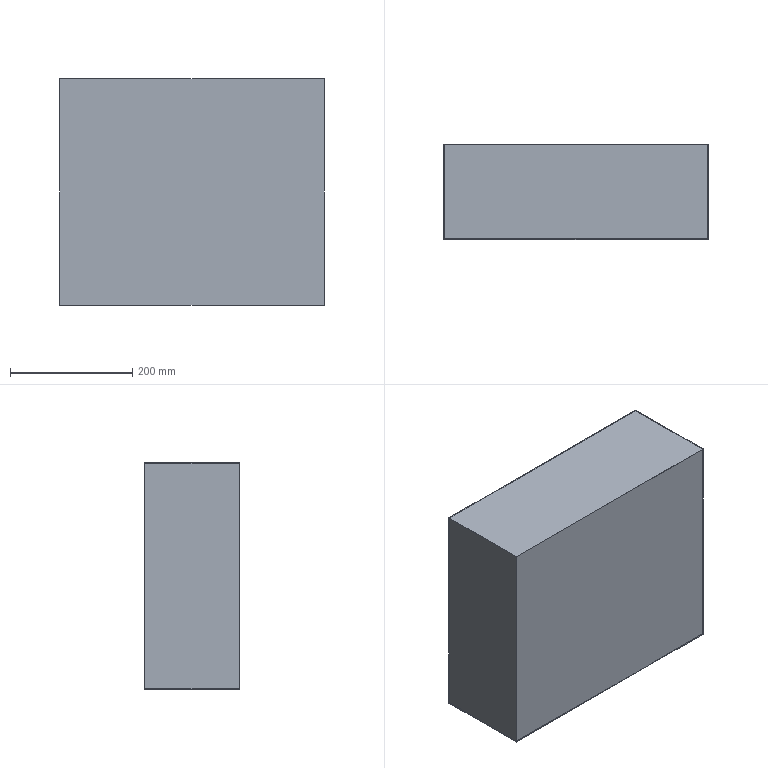Part | STEP file | STANDARD CONTRILLER | 1 solid | 12 faces | box 432 x 156 x 371 mm | volume 567252 mm3 | plane 12
STEP:
#1=CARTESIAN_POINT('',(-70.587,137.128,371.));
#2=VERTEX_POINT('',#1);
#3=CARTESIAN_POINT('',(-70.587,-18.872,371.));
#4=VERTEX_POINT('',#3);
#5=CARTESIAN_POINT('',(-70.587,136.128,371.));
#6=DIRECTION('',(0.,-1.,0.));
#7=VECTOR('',#6,1000.);
#8=LINE('',#5,#7);
#9=EDGE_CURVE('',#2,#4,#8,.T.);
#10=ORIENTED_EDGE('',*,*,#9,.T.);
#11=CARTESIAN_POINT('',(361.413,-18.872,371.));
#12=VERTEX_POINT('',#11);
#13=CARTESIAN_POINT('',(-69.587,-18.872,371.));
#14=DIRECTION('',(1.,0.,0.));
#15=VECTOR('',#14,1000.);
#16=LINE('',#13,#15);
#17=EDGE_CURVE('',#4,#12,#16,.T.);
#18=ORIENTED_EDGE('',*,*,#17,.T.);
#19=CARTESIAN_POINT('',(361.413,137.128,371.));
#20=VERTEX_POINT('',#19);
#21=CARTESIAN_POINT('',(361.413,136.128,371.));
#22=DIRECTION('',(0.,1.,0.));
#23=VECTOR('',#22,1000.);
#24=LINE('',#21,#23);
#25=EDGE_CURVE('',#12,#20,#24,.T.);
#26=ORIENTED_EDGE('',*,*,#25,.T.);
#27=CARTESIAN_POINT('',(-69.587,137.128,371.));
#28=DIRECTION('',(-1.,0.,0.));
#29=VECTOR('',#28,1000.);
#30=LINE('',#27,#29);
#31=EDGE_CURVE('',#20,#2,#30,.T.);
#32=ORIENTED_EDGE('',*,*,#31,.T.);
#33=EDGE_LOOP('',(#10,#18,#26,#32));
#34=FACE_OUTER_BOUND('',#33,.T.);
#35=CARTESIAN_POINT('',(-70.587,-18.872,371.));
#36=DIRECTION('',(0.,0.,1.));
#37=DIRECTION('',(1.,0.,0.));
#38=AXIS2_PLACEMENT_3D('',#35,#36,#37);
#39=PLANE('',#38);
#40=ADVANCED_FACE('',(#34),#39,.T.);
#41=CARTESIAN_POINT('',(-70.587,137.128,0.));
#42=VERTEX_POINT('',#41);
#43=CARTESIAN_POINT('',(-70.587,-18.872,0.));
#44=VERTEX_POINT('',#43);
#45=CARTESIAN_POINT('',(-70.587,136.128,0.));
#46=DIRECTION('',(0.,-1.,0.));
#47=VECTOR('',#46,1000.);
#48=LINE('',#45,#47);
#49=EDGE_CURVE('',#42,#44,#48,.T.);
#50=ORIENTED_EDGE('',*,*,#49,.F.);
#51=CARTESIAN_POINT('',(361.413,137.128,0.));
#52=VERTEX_POINT('',#51);
#53=CARTESIAN_POINT('',(-69.587,137.128,0.));
#54=DIRECTION('',(-1.,0.,0.));
#55=VECTOR('',#54,1000.);
#56=LINE('',#53,#55);
#57=EDGE_CURVE('',#52,#42,#56,.T.);
#58=ORIENTED_EDGE('',*,*,#57,.F.);
#59=CARTESIAN_POINT('',(361.413,-18.872,0.));
#60=VERTEX_POINT('',#59);
#61=CARTESIAN_POINT('',(361.413,136.128,0.));
#62=DIRECTION('',(0.,1.,0.));
#63=VECTOR('',#62,1000.);
#64=LINE('',#61,#63);
#65=EDGE_CURVE('',#60,#52,#64,.T.);
#66=ORIENTED_EDGE('',*,*,#65,.F.);
#67=CARTESIAN_POINT('',(-69.587,-18.872,0.));
#68=DIRECTION('',(1.,0.,0.));
#69=VECTOR('',#68,1000.);
#70=LINE('',#67,#69);
#71=EDGE_CURVE('',#44,#60,#70,.T.);
#72=ORIENTED_EDGE('',*,*,#71,.F.);
#73=EDGE_LOOP('',(#50,#58,#66,#72));
#74=FACE_OUTER_BOUND('',#73,.T.);
#75=CARTESIAN_POINT('',(-70.587,-18.872,0.));
#76=DIRECTION('',(0.,0.,1.));
#77=DIRECTION('',(1.,0.,0.));
#78=AXIS2_PLACEMENT_3D('',#75,#76,#77);
#79=PLANE('',#78);
#80=ADVANCED_FACE('',(#74),#79,.F.);
#81=ORIENTED_EDGE('',*,*,#49,.T.);
#82=CARTESIAN_POINT('',(-70.587,-18.872,371.));
#83=DIRECTION('',(0.,0.,-1.));
#84=VECTOR('',#83,1000.);
#85=LINE('',#82,#84);
#86=EDGE_CURVE('',#4,#44,#85,.T.);
#87=ORIENTED_EDGE('',*,*,#86,.F.);
#88=ORIENTED_EDGE('',*,*,#9,.F.);
#89=CARTESIAN_POINT('',(-70.587,137.128,371.));
#90=DIRECTION('',(0.,0.,-1.));
#91=VECTOR('',#90,1000.);
#92=LINE('',#89,#91);
#93=EDGE_CURVE('',#2,#42,#92,.T.);
#94=ORIENTED_EDGE('',*,*,#93,.T.);
#95=EDGE_LOOP('',(#81,#87,#88,#94));
#96=FACE_OUTER_BOUND('',#95,.T.);
#97=CARTESIAN_POINT('',(-70.587,136.128,371.));
#98=DIRECTION('',(1.,0.,0.));
#99=DIRECTION('',(0.,1.,0.));
#100=AXIS2_PLACEMENT_3D('',#97,#98,#99);
#101=PLANE('',#100);
#102=ADVANCED_FACE('',(#96),#101,.F.);
#103=ORIENTED_EDGE('',*,*,#71,.T.);
#104=CARTESIAN_POINT('',(361.413,-18.872,371.));
#105=DIRECTION('',(0.,0.,-1.));
#106=VECTOR('',#105,1000.);
#107=LINE('',#104,#106);
#108=EDGE_CURVE('',#12,#60,#107,.T.);
#109=ORIENTED_EDGE('',*,*,#108,.F.);
#110=ORIENTED_EDGE('',*,*,#17,.F.);
#111=ORIENTED_EDGE('',*,*,#86,.T.);
#112=EDGE_LOOP('',(#103,#109,#110,#111));
#113=FACE_OUTER_BOUND('',#112,.T.);
#114=CARTESIAN_POINT('',(-69.587,-18.872,371.));
#115=DIRECTION('',(0.,1.,0.));
#116=DIRECTION('',(0.,0.,1.));
#117=AXIS2_PLACEMENT_3D('',#114,#115,#116);
#118=PLANE('',#117);
#119=ADVANCED_FACE('',(#113),#118,.F.);
#120=ORIENTED_EDGE('',*,*,#65,.T.);
#121=CARTESIAN_POINT('',(361.413,137.128,371.));
#122=DIRECTION('',(0.,0.,-1.));
#123=VECTOR('',#122,1000.);
#124=LINE('',#121,#123);
#125=EDGE_CURVE('',#20,#52,#124,.T.);
#126=ORIENTED_EDGE('',*,*,#125,.F.);
#127=ORIENTED_EDGE('',*,*,#25,.F.);
#128=ORIENTED_EDGE('',*,*,#108,.T.);
#129=EDGE_LOOP('',(#120,#126,#127,#128));
#130=FACE_OUTER_BOUND('',#129,.T.);
#131=CARTESIAN_POINT('',(361.413,136.128,371.));
#132=DIRECTION('',(-1.,0.,0.));
#133=DIRECTION('',(0.,0.,1.));
#134=AXIS2_PLACEMENT_3D('',#131,#132,#133);
#135=PLANE('',#134);
#136=ADVANCED_FACE('',(#130),#135,.F.);
#137=ORIENTED_EDGE('',*,*,#57,.T.);
#138=ORIENTED_EDGE('',*,*,#93,.F.);
#139=ORIENTED_EDGE('',*,*,#31,.F.);
#140=ORIENTED_EDGE('',*,*,#125,.T.);
#141=EDGE_LOOP('',(#137,#138,#139,#140));
#142=FACE_OUTER_BOUND('',#141,.T.);
#143=CARTESIAN_POINT('',(-69.587,137.128,371.));
#144=DIRECTION('',(0.,-1.,0.));
#145=DIRECTION('',(0.,0.,-1.));
#146=AXIS2_PLACEMENT_3D('',#143,#144,#145);
#147=PLANE('',#146);
#148=ADVANCED_FACE('',(#142),#147,.F.);
#149=CLOSED_SHELL('',(#40,#80,#102,#119,#136,#148));
#150=CARTESIAN_POINT('',(360.413,136.128,1.));
#151=VERTEX_POINT('',#150);
#152=CARTESIAN_POINT('',(360.413,-17.872,1.));
#153=VERTEX_POINT('',#152);
#154=CARTESIAN_POINT('',(360.413,136.128,1.));
#155=DIRECTION('',(0.,-1.,0.));
#156=VECTOR('',#155,1000.);
#157=LINE('',#154,#156);
#158=EDGE_CURVE('',#151,#153,#157,.T.);
#159=ORIENTED_EDGE('',*,*,#158,.F.);
#160=CARTESIAN_POINT('',(-69.587,136.128,1.));
#161=VERTEX_POINT('',#160);
#162=CARTESIAN_POINT('',(360.413,136.128,1.));
#163=DIRECTION('',(1.,0.,0.));
#164=VECTOR('',#163,1000.);
#165=LINE('',#162,#164);
#166=EDGE_CURVE('',#161,#151,#165,.T.);
#167=ORIENTED_EDGE('',*,*,#166,.F.);
#168=CARTESIAN_POINT('',(-69.587,-17.872,1.));
#169=VERTEX_POINT('',#168);
#170=CARTESIAN_POINT('',(-69.587,136.128,1.));
#171=DIRECTION('',(0.,1.,0.));
#172=VECTOR('',#171,1000.);
#173=LINE('',#170,#172);
#174=EDGE_CURVE('',#169,#161,#173,.T.);
#175=ORIENTED_EDGE('',*,*,#174,.F.);
#176=CARTESIAN_POINT('',(360.413,-17.872,1.));
#177=DIRECTION('',(-1.,0.,0.));
#178=VECTOR('',#177,1000.);
#179=LINE('',#176,#178);
#180=EDGE_CURVE('',#153,#169,#179,.T.);
#181=ORIENTED_EDGE('',*,*,#180,.F.);
#182=EDGE_LOOP('',(#159,#167,#175,#181));
#183=FACE_OUTER_BOUND('',#182,.T.);
#184=CARTESIAN_POINT('',(360.413,-17.872,1.));
#185=DIRECTION('',(0.,0.,-1.));
#186=DIRECTION('',(-1.,0.,0.));
#187=AXIS2_PLACEMENT_3D('',#184,#185,#186);
#188=PLANE('',#187);
#189=ADVANCED_FACE('',(#183),#188,.F.);
#190=CARTESIAN_POINT('',(-69.587,136.128,370.));
#191=VERTEX_POINT('',#190);
#192=CARTESIAN_POINT('',(-69.587,-17.872,370.));
#193=VERTEX_POINT('',#192);
#194=CARTESIAN_POINT('',(-69.587,136.128,370.));
#195=DIRECTION('',(0.,-1.,0.));
#196=VECTOR('',#195,1000.);
#197=LINE('',#194,#196);
#198=EDGE_CURVE('',#191,#193,#197,.T.);
#199=ORIENTED_EDGE('',*,*,#198,.F.);
#200=CARTESIAN_POINT('',(360.413,136.128,370.));
#201=VERTEX_POINT('',#200);
#202=CARTESIAN_POINT('',(-69.587,136.128,370.));
#203=DIRECTION('',(-1.,0.,0.));
#204=VECTOR('',#203,1000.);
#205=LINE('',#202,#204);
#206=EDGE_CURVE('',#201,#191,#205,.T.);
#207=ORIENTED_EDGE('',*,*,#206,.F.);
#208=CARTESIAN_POINT('',(360.413,-17.872,370.));
#209=VERTEX_POINT('',#208);
#210=CARTESIAN_POINT('',(360.413,136.128,370.));
#211=DIRECTION('',(0.,1.,0.));
#212=VECTOR('',#211,1000.);
#213=LINE('',#210,#212);
#214=EDGE_CURVE('',#209,#201,#213,.T.);
#215=ORIENTED_EDGE('',*,*,#214,.F.);
#216=CARTESIAN_POINT('',(-69.587,-17.872,370.));
#217=DIRECTION('',(1.,0.,0.));
#218=VECTOR('',#217,1000.);
#219=LINE('',#216,#218);
#220=EDGE_CURVE('',#193,#209,#219,.T.);
#221=ORIENTED_EDGE('',*,*,#220,.F.);
#222=EDGE_LOOP('',(#199,#207,#215,#221));
#223=FACE_OUTER_BOUND('',#222,.T.);
#224=CARTESIAN_POINT('',(-69.587,-17.872,370.));
#225=DIRECTION('',(0.,0.,1.));
#226=DIRECTION('',(1.,0.,0.));
#227=AXIS2_PLACEMENT_3D('',#224,#225,#226);
#228=PLANE('',#227);
#229=ADVANCED_FACE('',(#223),#228,.F.);
#230=CARTESIAN_POINT('',(-69.587,136.128,371.));
#231=DIRECTION('',(0.,0.,-1.));
#232=VECTOR('',#231,1000.);
#233=LINE('',#230,#232);
#234=EDGE_CURVE('',#191,#161,#233,.T.);
#235=ORIENTED_EDGE('',*,*,#234,.T.);
#236=ORIENTED_EDGE('',*,*,#166,.T.);
#237=CARTESIAN_POINT('',(360.413,136.128,371.));
#238=DIRECTION('',(0.,0.,-1.));
#239=VECTOR('',#238,1000.);
#240=LINE('',#237,#239);
#241=EDGE_CURVE('',#201,#151,#240,.T.);
#242=ORIENTED_EDGE('',*,*,#241,.F.);
#243=ORIENTED_EDGE('',*,*,#206,.T.);
#244=EDGE_LOOP('',(#235,#236,#242,#243));
#245=FACE_OUTER_BOUND('',#244,.T.);
#246=CARTESIAN_POINT('',(-69.587,136.128,371.));
#247=DIRECTION('',(0.,-1.,0.));
#248=DIRECTION('',(0.,0.,-1.));
#249=AXIS2_PLACEMENT_3D('',#246,#247,#248);
#250=PLANE('',#249);
#251=ADVANCED_FACE('',(#245),#250,.T.);
#252=ORIENTED_EDGE('',*,*,#241,.T.);
#253=ORIENTED_EDGE('',*,*,#158,.T.);
#254=CARTESIAN_POINT('',(360.413,-17.872,371.));
#255=DIRECTION('',(0.,0.,-1.));
#256=VECTOR('',#255,1000.);
#257=LINE('',#254,#256);
#258=EDGE_CURVE('',#209,#153,#257,.T.);
#259=ORIENTED_EDGE('',*,*,#258,.F.);
#260=ORIENTED_EDGE('',*,*,#214,.T.);
#261=EDGE_LOOP('',(#252,#253,#259,#260));
#262=FACE_OUTER_BOUND('',#261,.T.);
#263=CARTESIAN_POINT('',(360.413,136.128,371.));
#264=DIRECTION('',(-1.,0.,0.));
#265=DIRECTION('',(0.,0.,1.));
#266=AXIS2_PLACEMENT_3D('',#263,#264,#265);
#267=PLANE('',#266);
#268=ADVANCED_FACE('',(#262),#267,.T.);
#269=ORIENTED_EDGE('',*,*,#258,.T.);
#270=ORIENTED_EDGE('',*,*,#180,.T.);
#271=CARTESIAN_POINT('',(-69.587,-17.872,371.));
#272=DIRECTION('',(0.,0.,-1.));
#273=VECTOR('',#272,1000.);
#274=LINE('',#271,#273);
#275=EDGE_CURVE('',#193,#169,#274,.T.);
#276=ORIENTED_EDGE('',*,*,#275,.F.);
#277=ORIENTED_EDGE('',*,*,#220,.T.);
#278=EDGE_LOOP('',(#269,#270,#276,#277));
#279=FACE_OUTER_BOUND('',#278,.T.);
#280=CARTESIAN_POINT('',(-69.587,-17.872,371.));
#281=DIRECTION('',(0.,1.,0.));
#282=DIRECTION('',(0.,0.,1.));
#283=AXIS2_PLACEMENT_3D('',#280,#281,#282);
#284=PLANE('',#283);
#285=ADVANCED_FACE('',(#279),#284,.T.);
#286=ORIENTED_EDGE('',*,*,#275,.T.);
#287=ORIENTED_EDGE('',*,*,#174,.T.);
#288=ORIENTED_EDGE('',*,*,#234,.F.);
#289=ORIENTED_EDGE('',*,*,#198,.T.);
#290=EDGE_LOOP('',(#286,#287,#288,#289));
#291=FACE_OUTER_BOUND('',#290,.T.);
#292=CARTESIAN_POINT('',(-69.587,136.128,371.));
#293=DIRECTION('',(1.,0.,0.));
#294=DIRECTION('',(0.,1.,0.));
#295=AXIS2_PLACEMENT_3D('',#292,#293,#294);
#296=PLANE('',#295);
#297=ADVANCED_FACE('',(#291),#296,.T.);
#298=CLOSED_SHELL('',(#189,#229,#251,#268,#285,#297));
#299=ORIENTED_CLOSED_SHELL('',*,#298,.F.);
#300=BREP_WITH_VOIDS('',#149,(#299));
#301=CARTESIAN_POINT('',(0.,0.,0.));
#302=DIRECTION('',(0.,0.,1.));
#303=DIRECTION('',(1.,0.,0.));
#304=AXIS2_PLACEMENT_3D('',#301,#302,#303);
#305=(LENGTH_UNIT()NAMED_UNIT(*)SI_UNIT(.MILLI.,.METRE.));
#306=UNCERTAINTY_MEASURE_WITH_UNIT(LENGTH_MEASURE(0.00001),#305,'','');
#307=(NAMED_UNIT(*)PLANE_ANGLE_UNIT()SI_UNIT($,.RADIAN.));
#308=(NAMED_UNIT(*)SI_UNIT($,.STERADIAN.)SOLID_ANGLE_UNIT());
#309=(GEOMETRIC_REPRESENTATION_CONTEXT(3)GLOBAL_UNCERTAINTY_ASSIGNED_CONTEXT((#306))GLOBAL_UNIT_ASSIGNED_CONTEXT((#305,#307,#308))REPRESENTATION_CONTEXT('',''));
#310=ADVANCED_BREP_SHAPE_REPRESENTATION('',(#300,#304),#309);